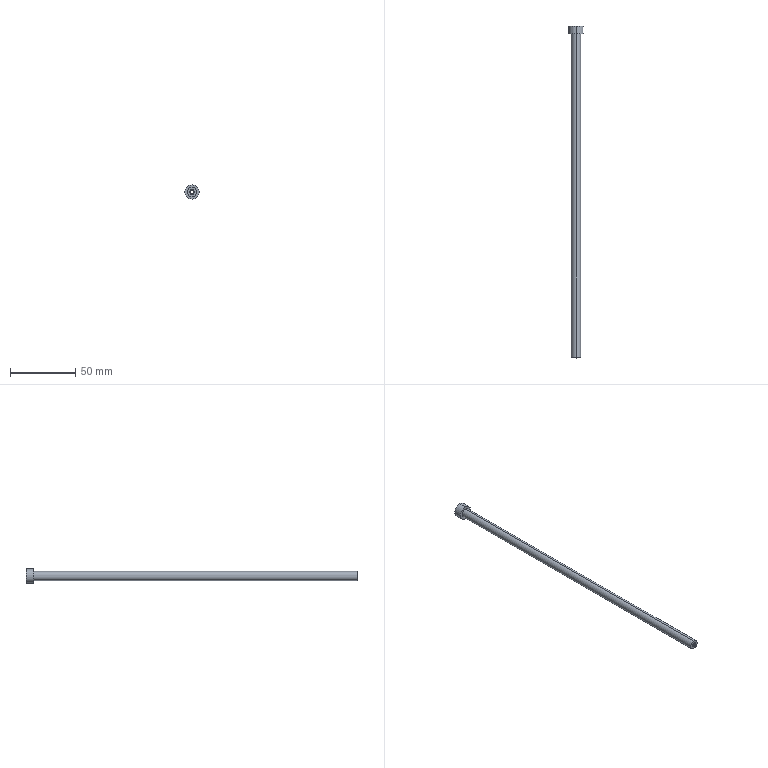Part | STEP file | 1 solid | 13 faces | box 11 x 254.534 x 11 mm | volume 8863 mm3 | cylinder 6 | cone 4 | plane 3 | commonest cylinder face diameters 2.5 x2 7 x2 11 x2
STEP:
#1=CARTESIAN_POINT('',(0.,0.,0.));
#2=DIRECTION('',(0.,0.,1.));
#3=DIRECTION('',(1.,0.,0.));
#4=AXIS2_PLACEMENT_3D('',#1,#2,#3);
#5=CARTESIAN_POINT('',(-16.582,290.5,177.41));
#6=VERTEX_POINT('',#5);
#7=CARTESIAN_POINT('',(-16.582,290.5,188.41));
#8=VERTEX_POINT('',#7);
#9=CARTESIAN_POINT('',(-16.582,290.5,182.91));
#10=DIRECTION('',(0.,-1.,0.));
#11=DIRECTION('',(0.,0.,-1.));
#12=AXIS2_PLACEMENT_3D('',#9,#10,#11);
#13=CIRCLE('',#12,5.5);
#14=CARTESIAN_POINT('',(-16.582,290.5,182.91));
#15=DIRECTION('',(0.,-1.,0.));
#16=DIRECTION('',(0.,0.,-1.));
#17=AXIS2_PLACEMENT_3D('',#14,#15,#16);
#18=CYLINDRICAL_SURFACE('',#17,5.5);
#19=CARTESIAN_POINT('',(0.,0.));
#20=DIRECTION('',(1.,0.));
#21=VECTOR('',#20,1.);
#22=LINE('',#19,#21);
#23=(GEOMETRIC_REPRESENTATION_CONTEXT(2)PARAMETRIC_REPRESENTATION_CONTEXT()REPRESENTATION_CONTEXT('',''));
#24=DEFINITIONAL_REPRESENTATION('',(#22),#23);
#25=PCURVE('',#18,#24);
#26=CARTESIAN_POINT('',(-72.862,290.5,110.196));
#27=DIRECTION('',(0.,-1.,0.));
#28=DIRECTION('',(0.,0.,-1.));
#29=AXIS2_PLACEMENT_3D('',#26,#27,#28);
#30=PLANE('',#29);
#31=CARTESIAN_POINT('',(-72.714,56.28));
#32=DIRECTION('',(1.,0.));
#33=AXIS2_PLACEMENT_2D('',#31,#32);
#34=CIRCLE('',#33,5.5);
#35=(GEOMETRIC_REPRESENTATION_CONTEXT(2)PARAMETRIC_REPRESENTATION_CONTEXT()REPRESENTATION_CONTEXT('',''));
#36=DEFINITIONAL_REPRESENTATION('',(#34),#35);
#37=PCURVE('',#30,#36);
#38=SURFACE_CURVE('',#13,(#25,#37),.PCURVE_S1.);
#39=EDGE_CURVE('',#6,#8,#38,.T.);
#40=ORIENTED_EDGE('',*,*,#39,.T.);
#41=CARTESIAN_POINT('',(-16.582,284.5,188.41));
#42=VERTEX_POINT('',#41);
#43=CARTESIAN_POINT('',(-16.582,290.5,188.41));
#44=DIRECTION('',(0.,-1.,0.));
#45=VECTOR('',#44,1.);
#46=LINE('',#43,#45);
#47=CARTESIAN_POINT('',(3.142,0.));
#48=DIRECTION('',(0.,1.));
#49=VECTOR('',#48,1.);
#50=LINE('',#47,#49);
#51=(GEOMETRIC_REPRESENTATION_CONTEXT(2)PARAMETRIC_REPRESENTATION_CONTEXT()REPRESENTATION_CONTEXT('',''));
#52=DEFINITIONAL_REPRESENTATION('',(#50),#51);
#53=PCURVE('',#18,#52);
#54=CARTESIAN_POINT('',(-16.582,290.5,182.91));
#55=DIRECTION('',(0.,-1.,0.));
#56=DIRECTION('',(0.,0.,-1.));
#57=AXIS2_PLACEMENT_3D('',#54,#55,#56);
#58=CYLINDRICAL_SURFACE('',#57,5.5);
#59=CARTESIAN_POINT('',(3.142,0.));
#60=DIRECTION('',(0.,1.));
#61=VECTOR('',#60,1.);
#62=LINE('',#59,#61);
#63=(GEOMETRIC_REPRESENTATION_CONTEXT(2)PARAMETRIC_REPRESENTATION_CONTEXT()REPRESENTATION_CONTEXT('',''));
#64=DEFINITIONAL_REPRESENTATION('',(#62),#63);
#65=PCURVE('',#58,#64);
#66=SURFACE_CURVE('',#46,(#53,#65),.PCURVE_S1.);
#67=EDGE_CURVE('',#8,#42,#66,.T.);
#68=ORIENTED_EDGE('',*,*,#67,.T.);
#69=CARTESIAN_POINT('',(-16.582,284.5,177.41));
#70=VERTEX_POINT('',#69);
#71=CARTESIAN_POINT('',(-16.582,284.5,182.91));
#72=DIRECTION('',(0.,1.,0.));
#73=DIRECTION('',(0.,0.,1.));
#74=AXIS2_PLACEMENT_3D('',#71,#72,#73);
#75=CIRCLE('',#74,5.5);
#76=CARTESIAN_POINT('',(3.142,6.));
#77=DIRECTION('',(-1.,0.));
#78=VECTOR('',#77,1.);
#79=LINE('',#76,#78);
#80=(GEOMETRIC_REPRESENTATION_CONTEXT(2)PARAMETRIC_REPRESENTATION_CONTEXT()REPRESENTATION_CONTEXT('',''));
#81=DEFINITIONAL_REPRESENTATION('',(#79),#80);
#82=PCURVE('',#18,#81);
#83=CARTESIAN_POINT('',(-16.582,284.5,182.91));
#84=DIRECTION('',(0.,-1.,0.));
#85=DIRECTION('',(0.,0.,-1.));
#86=AXIS2_PLACEMENT_3D('',#83,#84,#85);
#87=PLANE('',#86);
#88=CARTESIAN_POINT('',(-5.5,0.));
#89=CARTESIAN_POINT('',(-5.5,9.526));
#90=CARTESIAN_POINT('',(2.75,4.763));
#91=CARTESIAN_POINT('',(11.,0.));
#92=CARTESIAN_POINT('',(2.75,-4.763));
#93=CARTESIAN_POINT('',(-5.5,-9.526));
#94=CARTESIAN_POINT('',(-5.5,0.));
#95=(BOUNDED_CURVE()B_SPLINE_CURVE(2,(#88,#89,#90,#91,#92,#93,#94),.UNSPECIFIED.,.T.,.F.)B_SPLINE_CURVE_WITH_KNOTS((1,2,2,2,2,1),(-2.094,0.,2.094,4.189,6.283,8.378),.UNSPECIFIED.)CURVE()GEOMETRIC_REPRESENTATION_ITEM()RATIONAL_B_SPLINE_CURVE((1.,0.5,1.,0.5,1.,0.5,1.))REPRESENTATION_ITEM(''));
#96=(GEOMETRIC_REPRESENTATION_CONTEXT(2)PARAMETRIC_REPRESENTATION_CONTEXT()REPRESENTATION_CONTEXT('',''));
#97=DEFINITIONAL_REPRESENTATION('',(#95),#96);
#98=PCURVE('',#87,#97);
#99=SURFACE_CURVE('',#75,(#82,#98),.PCURVE_S1.);
#100=EDGE_CURVE('',#42,#70,#99,.T.);
#101=ORIENTED_EDGE('',*,*,#100,.T.);
#102=CARTESIAN_POINT('',(-16.582,290.5,177.41));
#103=DIRECTION('',(0.,-1.,0.));
#104=VECTOR('',#103,1.);
#105=LINE('',#102,#104);
#106=CARTESIAN_POINT('',(0.,0.));
#107=DIRECTION('',(0.,1.));
#108=VECTOR('',#107,1.);
#109=LINE('',#106,#108);
#110=(GEOMETRIC_REPRESENTATION_CONTEXT(2)PARAMETRIC_REPRESENTATION_CONTEXT()REPRESENTATION_CONTEXT('',''));
#111=DEFINITIONAL_REPRESENTATION('',(#109),#110);
#112=PCURVE('',#18,#111);
#113=CARTESIAN_POINT('',(6.283,0.));
#114=DIRECTION('',(0.,1.));
#115=VECTOR('',#114,1.);
#116=LINE('',#113,#115);
#117=(GEOMETRIC_REPRESENTATION_CONTEXT(2)PARAMETRIC_REPRESENTATION_CONTEXT()REPRESENTATION_CONTEXT('',''));
#118=DEFINITIONAL_REPRESENTATION('',(#116),#117);
#119=PCURVE('',#58,#118);
#120=SURFACE_CURVE('',#105,(#112,#119),.PCURVE_S1.);
#121=EDGE_CURVE('',#6,#70,#120,.T.);
#122=ORIENTED_EDGE('',*,*,#121,.F.);
#123=EDGE_LOOP('',(#40,#68,#101,#122));
#124=FACE_BOUND('',#123,.T.);
#125=ADVANCED_FACE('',(#124),#18,.T.);
#126=CARTESIAN_POINT('',(-16.582,35.966,184.16));
#127=VERTEX_POINT('',#126);
#128=CARTESIAN_POINT('',(-16.582,290.5,184.16));
#129=VERTEX_POINT('',#128);
#130=CARTESIAN_POINT('',(-16.582,27.637,184.16));
#131=DIRECTION('',(0.,1.,0.));
#132=VECTOR('',#131,1.);
#133=LINE('',#130,#132);
#134=CARTESIAN_POINT('',(-16.582,27.637,182.91));
#135=DIRECTION('',(0.,1.,0.));
#136=DIRECTION('',(0.,0.,1.));
#137=AXIS2_PLACEMENT_3D('',#134,#135,#136);
#138=CYLINDRICAL_SURFACE('',#137,1.25);
#139=CARTESIAN_POINT('',(6.283,0.));
#140=DIRECTION('',(0.,1.));
#141=VECTOR('',#140,1.);
#142=LINE('',#139,#141);
#143=(GEOMETRIC_REPRESENTATION_CONTEXT(2)PARAMETRIC_REPRESENTATION_CONTEXT()REPRESENTATION_CONTEXT('',''));
#144=DEFINITIONAL_REPRESENTATION('',(#142),#143);
#145=PCURVE('',#138,#144);
#146=CARTESIAN_POINT('',(-16.582,27.637,182.91));
#147=DIRECTION('',(0.,1.,0.));
#148=DIRECTION('',(0.,0.,1.));
#149=AXIS2_PLACEMENT_3D('',#146,#147,#148);
#150=CYLINDRICAL_SURFACE('',#149,1.25);
#151=CARTESIAN_POINT('',(0.,0.));
#152=DIRECTION('',(0.,1.));
#153=VECTOR('',#152,1.);
#154=LINE('',#151,#153);
#155=(GEOMETRIC_REPRESENTATION_CONTEXT(2)PARAMETRIC_REPRESENTATION_CONTEXT()REPRESENTATION_CONTEXT('',''));
#156=DEFINITIONAL_REPRESENTATION('',(#154),#155);
#157=PCURVE('',#150,#156);
#158=SURFACE_CURVE('',#133,(#145,#157),.PCURVE_S1.);
#159=EDGE_CURVE('',#127,#129,#158,.T.);
#160=ORIENTED_EDGE('',*,*,#159,.T.);
#161=CARTESIAN_POINT('',(-16.582,290.5,181.66));
#162=VERTEX_POINT('',#161);
#163=CARTESIAN_POINT('',(-16.582,290.5,182.91));
#164=DIRECTION('',(0.,-1.,0.));
#165=DIRECTION('',(0.,0.,-1.));
#166=AXIS2_PLACEMENT_3D('',#163,#164,#165);
#167=CIRCLE('',#166,1.25);
#168=CARTESIAN_POINT('',(9.425,262.863));
#169=DIRECTION('',(-1.,0.));
#170=VECTOR('',#169,1.);
#171=LINE('',#168,#170);
#172=(GEOMETRIC_REPRESENTATION_CONTEXT(2)PARAMETRIC_REPRESENTATION_CONTEXT()REPRESENTATION_CONTEXT('',''));
#173=DEFINITIONAL_REPRESENTATION('',(#171),#172);
#174=PCURVE('',#138,#173);
#175=CARTESIAN_POINT('',(-72.714,56.28));
#176=DIRECTION('',(1.,0.));
#177=AXIS2_PLACEMENT_2D('',#175,#176);
#178=CIRCLE('',#177,1.25);
#179=(GEOMETRIC_REPRESENTATION_CONTEXT(2)PARAMETRIC_REPRESENTATION_CONTEXT()REPRESENTATION_CONTEXT('',''));
#180=DEFINITIONAL_REPRESENTATION('',(#178),#179);
#181=PCURVE('',#30,#180);
#182=SURFACE_CURVE('',#167,(#174,#181),.PCURVE_S1.);
#183=EDGE_CURVE('',#129,#162,#182,.T.);
#184=ORIENTED_EDGE('',*,*,#183,.T.);
#185=CARTESIAN_POINT('',(-16.582,35.966,181.66));
#186=VERTEX_POINT('',#185);
#187=CARTESIAN_POINT('',(-16.582,27.637,181.66));
#188=DIRECTION('',(0.,1.,0.));
#189=VECTOR('',#188,1.);
#190=LINE('',#187,#189);
#191=CARTESIAN_POINT('',(3.142,0.));
#192=DIRECTION('',(0.,1.));
#193=VECTOR('',#192,1.);
#194=LINE('',#191,#193);
#195=(GEOMETRIC_REPRESENTATION_CONTEXT(2)PARAMETRIC_REPRESENTATION_CONTEXT()REPRESENTATION_CONTEXT('',''));
#196=DEFINITIONAL_REPRESENTATION('',(#194),#195);
#197=PCURVE('',#138,#196);
#198=CARTESIAN_POINT('',(3.142,0.));
#199=DIRECTION('',(0.,1.));
#200=VECTOR('',#199,1.);
#201=LINE('',#198,#200);
#202=(GEOMETRIC_REPRESENTATION_CONTEXT(2)PARAMETRIC_REPRESENTATION_CONTEXT()REPRESENTATION_CONTEXT('',''));
#203=DEFINITIONAL_REPRESENTATION('',(#201),#202);
#204=PCURVE('',#150,#203);
#205=SURFACE_CURVE('',#190,(#197,#204),.PCURVE_S1.);
#206=EDGE_CURVE('',#186,#162,#205,.T.);
#207=ORIENTED_EDGE('',*,*,#206,.F.);
#208=CARTESIAN_POINT('',(-16.582,35.966,182.91));
#209=DIRECTION('',(0.,1.,0.));
#210=DIRECTION('',(0.,0.,1.));
#211=AXIS2_PLACEMENT_3D('',#208,#209,#210);
#212=CIRCLE('',#211,1.25);
#213=CARTESIAN_POINT('',(0.,8.329));
#214=DIRECTION('',(1.,0.));
#215=VECTOR('',#214,1.);
#216=LINE('',#213,#215);
#217=(GEOMETRIC_REPRESENTATION_CONTEXT(2)PARAMETRIC_REPRESENTATION_CONTEXT()REPRESENTATION_CONTEXT('',''));
#218=DEFINITIONAL_REPRESENTATION('',(#216),#217);
#219=PCURVE('',#138,#218);
#220=CARTESIAN_POINT('',(-16.582,36.682,182.91));
#221=DIRECTION('',(0.,1.,0.));
#222=DIRECTION('',(0.,0.,1.));
#223=AXIS2_PLACEMENT_3D('',#220,#221,#222);
#224=CONICAL_SURFACE('',#223,1.256,0.008727);
#225=CARTESIAN_POINT('',(0.,-0.7162));
#226=DIRECTION('',(1.,0.));
#227=VECTOR('',#226,1.);
#228=LINE('',#225,#227);
#229=(GEOMETRIC_REPRESENTATION_CONTEXT(2)PARAMETRIC_REPRESENTATION_CONTEXT()REPRESENTATION_CONTEXT('',''));
#230=DEFINITIONAL_REPRESENTATION('',(#228),#229);
#231=PCURVE('',#224,#230);
#232=SURFACE_CURVE('',#212,(#219,#231),.PCURVE_S1.);
#233=EDGE_CURVE('',#186,#127,#232,.T.);
#234=ORIENTED_EDGE('',*,*,#233,.T.);
#235=EDGE_LOOP('',(#160,#184,#207,#234));
#236=FACE_BOUND('',#235,.F.);
#237=ADVANCED_FACE('',(#236),#138,.F.);
#238=CARTESIAN_POINT('',(-16.582,36.682,179.41));
#239=VERTEX_POINT('',#238);
#240=CARTESIAN_POINT('',(-16.582,36.682,186.41));
#241=VERTEX_POINT('',#240);
#242=CARTESIAN_POINT('',(-16.582,36.682,182.91));
#243=DIRECTION('',(0.,-1.,0.));
#244=DIRECTION('',(0.,0.,1.));
#245=AXIS2_PLACEMENT_3D('',#242,#243,#244);
#246=CIRCLE('',#245,3.5);
#247=CARTESIAN_POINT('',(-16.582,27.637,182.91));
#248=DIRECTION('',(0.,1.,0.));
#249=DIRECTION('',(0.,0.,1.));
#250=AXIS2_PLACEMENT_3D('',#247,#248,#249);
#251=CYLINDRICAL_SURFACE('',#250,3.5);
#252=CARTESIAN_POINT('',(6.283,9.045));
#253=DIRECTION('',(-1.,0.));
#254=VECTOR('',#253,1.);
#255=LINE('',#252,#254);
#256=(GEOMETRIC_REPRESENTATION_CONTEXT(2)PARAMETRIC_REPRESENTATION_CONTEXT()REPRESENTATION_CONTEXT('',''));
#257=DEFINITIONAL_REPRESENTATION('',(#255),#256);
#258=PCURVE('',#251,#257);
#259=CARTESIAN_POINT('',(-16.582,36.682,182.91));
#260=DIRECTION('',(0.,1.,0.));
#261=DIRECTION('',(0.,0.,1.));
#262=AXIS2_PLACEMENT_3D('',#259,#260,#261);
#263=PLANE('',#262);
#264=CARTESIAN_POINT('',(3.5,0.));
#265=CARTESIAN_POINT('',(3.5,-6.062));
#266=CARTESIAN_POINT('',(-1.75,-3.031));
#267=CARTESIAN_POINT('',(-7.,0.));
#268=CARTESIAN_POINT('',(-1.75,3.031));
#269=CARTESIAN_POINT('',(3.5,6.062));
#270=CARTESIAN_POINT('',(3.5,0.));
#271=(BOUNDED_CURVE()B_SPLINE_CURVE(2,(#264,#265,#266,#267,#268,#269,#270),.UNSPECIFIED.,.T.,.F.)B_SPLINE_CURVE_WITH_KNOTS((1,2,2,2,2,1),(-2.094,0.,2.094,4.189,6.283,8.378),.UNSPECIFIED.)CURVE()GEOMETRIC_REPRESENTATION_ITEM()RATIONAL_B_SPLINE_CURVE((1.,0.5,1.,0.5,1.,0.5,1.))REPRESENTATION_ITEM(''));
#272=(GEOMETRIC_REPRESENTATION_CONTEXT(2)PARAMETRIC_REPRESENTATION_CONTEXT()REPRESENTATION_CONTEXT('',''));
#273=DEFINITIONAL_REPRESENTATION('',(#271),#272);
#274=PCURVE('',#263,#273);
#275=SURFACE_CURVE('',#246,(#258,#274),.PCURVE_S1.);
#276=EDGE_CURVE('',#239,#241,#275,.T.);
#277=ORIENTED_EDGE('',*,*,#276,.F.);
#278=CARTESIAN_POINT('',(-16.582,284.5,179.41));
#279=VERTEX_POINT('',#278);
#280=CARTESIAN_POINT('',(-16.582,27.637,179.41));
#281=DIRECTION('',(0.,1.,0.));
#282=VECTOR('',#281,1.);
#283=LINE('',#280,#282);
#284=CARTESIAN_POINT('',(3.142,0.));
#285=DIRECTION('',(0.,1.));
#286=VECTOR('',#285,1.);
#287=LINE('',#284,#286);
#288=(GEOMETRIC_REPRESENTATION_CONTEXT(2)PARAMETRIC_REPRESENTATION_CONTEXT()REPRESENTATION_CONTEXT('',''));
#289=DEFINITIONAL_REPRESENTATION('',(#287),#288);
#290=PCURVE('',#251,#289);
#291=CARTESIAN_POINT('',(-16.582,27.637,182.91));
#292=DIRECTION('',(0.,1.,0.));
#293=DIRECTION('',(0.,0.,1.));
#294=AXIS2_PLACEMENT_3D('',#291,#292,#293);
#295=CYLINDRICAL_SURFACE('',#294,3.5);
#296=CARTESIAN_POINT('',(3.142,0.));
#297=DIRECTION('',(0.,1.));
#298=VECTOR('',#297,1.);
#299=LINE('',#296,#298);
#300=(GEOMETRIC_REPRESENTATION_CONTEXT(2)PARAMETRIC_REPRESENTATION_CONTEXT()REPRESENTATION_CONTEXT('',''));
#301=DEFINITIONAL_REPRESENTATION('',(#299),#300);
#302=PCURVE('',#295,#301);
#303=SURFACE_CURVE('',#283,(#290,#302),.PCURVE_S1.);
#304=EDGE_CURVE('',#239,#279,#303,.T.);
#305=ORIENTED_EDGE('',*,*,#304,.T.);
#306=CARTESIAN_POINT('',(-16.582,284.5,186.41));
#307=VERTEX_POINT('',#306);
#308=CARTESIAN_POINT('',(-16.582,284.5,182.91));
#309=DIRECTION('',(0.,1.,0.));
#310=DIRECTION('',(0.,0.,-1.));
#311=AXIS2_PLACEMENT_3D('',#308,#309,#310);
#312=CIRCLE('',#311,3.5);
#313=CARTESIAN_POINT('',(-3.142,256.863));
#314=DIRECTION('',(1.,0.));
#315=VECTOR('',#314,1.);
#316=LINE('',#313,#315);
#317=(GEOMETRIC_REPRESENTATION_CONTEXT(2)PARAMETRIC_REPRESENTATION_CONTEXT()REPRESENTATION_CONTEXT('',''));
#318=DEFINITIONAL_REPRESENTATION('',(#316),#317);
#319=PCURVE('',#251,#318);
#320=CARTESIAN_POINT('',(3.5,0.));
#321=CARTESIAN_POINT('',(3.5,-6.062));
#322=CARTESIAN_POINT('',(-1.75,-3.031));
#323=CARTESIAN_POINT('',(-7.,0.));
#324=CARTESIAN_POINT('',(-1.75,3.031));
#325=CARTESIAN_POINT('',(3.5,6.062));
#326=CARTESIAN_POINT('',(3.5,0.));
#327=(BOUNDED_CURVE()B_SPLINE_CURVE(2,(#320,#321,#322,#323,#324,#325,#326),.UNSPECIFIED.,.T.,.F.)B_SPLINE_CURVE_WITH_KNOTS((1,2,2,2,2,1),(-2.094,0.,2.094,4.189,6.283,8.378),.UNSPECIFIED.)CURVE()GEOMETRIC_REPRESENTATION_ITEM()RATIONAL_B_SPLINE_CURVE((1.,0.5,1.,0.5,1.,0.5,1.))REPRESENTATION_ITEM(''));
#328=(GEOMETRIC_REPRESENTATION_CONTEXT(2)PARAMETRIC_REPRESENTATION_CONTEXT()REPRESENTATION_CONTEXT('',''));
#329=DEFINITIONAL_REPRESENTATION('',(#327),#328);
#330=PCURVE('',#87,#329);
#331=SURFACE_CURVE('',#312,(#319,#330),.PCURVE_S1.);
#332=EDGE_CURVE('',#307,#279,#331,.T.);
#333=ORIENTED_EDGE('',*,*,#332,.F.);
#334=CARTESIAN_POINT('',(-16.582,27.637,186.41));
#335=DIRECTION('',(0.,1.,0.));
#336=VECTOR('',#335,1.);
#337=LINE('',#334,#336);
#338=CARTESIAN_POINT('',(0.,0.));
#339=DIRECTION('',(0.,1.));
#340=VECTOR('',#339,1.);
#341=LINE('',#338,#340);
#342=(GEOMETRIC_REPRESENTATION_CONTEXT(2)PARAMETRIC_REPRESENTATION_CONTEXT()REPRESENTATION_CONTEXT('',''));
#343=DEFINITIONAL_REPRESENTATION('',(#341),#342);
#344=PCURVE('',#251,#343);
#345=CARTESIAN_POINT('',(6.283,0.));
#346=DIRECTION('',(0.,1.));
#347=VECTOR('',#346,1.);
#348=LINE('',#345,#347);
#349=(GEOMETRIC_REPRESENTATION_CONTEXT(2)PARAMETRIC_REPRESENTATION_CONTEXT()REPRESENTATION_CONTEXT('',''));
#350=DEFINITIONAL_REPRESENTATION('',(#348),#349);
#351=PCURVE('',#295,#350);
#352=SURFACE_CURVE('',#337,(#344,#351),.PCURVE_S1.);
#353=EDGE_CURVE('',#241,#307,#352,.T.);
#354=ORIENTED_EDGE('',*,*,#353,.F.);
#355=EDGE_LOOP('',(#277,#305,#333,#354));
#356=FACE_BOUND('',#355,.T.);
#357=ADVANCED_FACE('',(#356),#251,.T.);
#358=CARTESIAN_POINT('',(-16.582,36.176,184.162));
#359=VERTEX_POINT('',#358);
#360=CARTESIAN_POINT('',(-16.582,36.176,181.658));
#361=VERTEX_POINT('',#360);
#362=CARTESIAN_POINT('',(-16.582,36.176,182.91));
#363=DIRECTION('',(0.,1.,0.));
#364=DIRECTION('',(0.,0.,1.));
#365=AXIS2_PLACEMENT_3D('',#362,#363,#364);
#366=CIRCLE('',#365,1.252);
#367=CARTESIAN_POINT('',(-16.582,36.176,182.91));
#368=DIRECTION('',(0.,1.,0.));
#369=DIRECTION('',(0.,0.,1.));
#370=AXIS2_PLACEMENT_3D('',#367,#368,#369);
#371=CONICAL_SURFACE('',#370,1.252,0.7854);
#372=CARTESIAN_POINT('',(0.,0.));
#373=DIRECTION('',(1.,0.));
#374=VECTOR('',#373,1.);
#375=LINE('',#372,#374);
#376=(GEOMETRIC_REPRESENTATION_CONTEXT(2)PARAMETRIC_REPRESENTATION_CONTEXT()REPRESENTATION_CONTEXT('',''));
#377=DEFINITIONAL_REPRESENTATION('',(#375),#376);
#378=PCURVE('',#371,#377);
#379=CARTESIAN_POINT('',(-16.582,36.682,182.91));
#380=DIRECTION('',(0.,1.,0.));
#381=DIRECTION('',(0.,0.,1.));
#382=AXIS2_PLACEMENT_3D('',#379,#380,#381);
#383=CONICAL_SURFACE('',#382,1.256,0.008727);
#384=CARTESIAN_POINT('',(0.,-0.5069));
#385=DIRECTION('',(1.,0.));
#386=VECTOR('',#385,1.);
#387=LINE('',#384,#386);
#388=(GEOMETRIC_REPRESENTATION_CONTEXT(2)PARAMETRIC_REPRESENTATION_CONTEXT()REPRESENTATION_CONTEXT('',''));
#389=DEFINITIONAL_REPRESENTATION('',(#387),#388);
#390=PCURVE('',#383,#389);
#391=SURFACE_CURVE('',#366,(#378,#390),.PCURVE_S1.);
#392=EDGE_CURVE('',#359,#361,#391,.T.);
#393=ORIENTED_EDGE('',*,*,#392,.T.);
#394=CARTESIAN_POINT('',(-16.582,36.682,181.151));
#395=VERTEX_POINT('',#394);
#396=CARTESIAN_POINT('',(-16.582,36.176,181.658));
#397=DIRECTION('',(0.,0.7071,-0.7071));
#398=VECTOR('',#397,1.);
#399=LINE('',#396,#398);
#400=CARTESIAN_POINT('',(3.142,0.));
#401=DIRECTION('',(0.,1.));
#402=VECTOR('',#401,1.);
#403=LINE('',#400,#402);
#404=(GEOMETRIC_REPRESENTATION_CONTEXT(2)PARAMETRIC_REPRESENTATION_CONTEXT()REPRESENTATION_CONTEXT('',''));
#405=DEFINITIONAL_REPRESENTATION('',(#403),#404);
#406=PCURVE('',#371,#405);
#407=CARTESIAN_POINT('',(-16.582,36.176,182.91));
#408=DIRECTION('',(0.,1.,0.));
#409=DIRECTION('',(0.,0.,1.));
#410=AXIS2_PLACEMENT_3D('',#407,#408,#409);
#411=CONICAL_SURFACE('',#410,1.252,0.7854);
#412=CARTESIAN_POINT('',(3.142,0.));
#413=DIRECTION('',(0.,1.));
#414=VECTOR('',#413,1.);
#415=LINE('',#412,#414);
#416=(GEOMETRIC_REPRESENTATION_CONTEXT(2)PARAMETRIC_REPRESENTATION_CONTEXT()REPRESENTATION_CONTEXT('',''));
#417=DEFINITIONAL_REPRESENTATION('',(#415),#416);
#418=PCURVE('',#411,#417);
#419=SURFACE_CURVE('',#399,(#406,#418),.PCURVE_S1.);
#420=EDGE_CURVE('',#361,#395,#419,.T.);
#421=ORIENTED_EDGE('',*,*,#420,.T.);
#422=CARTESIAN_POINT('',(-16.582,36.682,184.669));
#423=VERTEX_POINT('',#422);
#424=CARTESIAN_POINT('',(-16.582,36.682,182.91));
#425=DIRECTION('',(0.,-1.,0.));
#426=DIRECTION('',(0.,0.,1.));
#427=AXIS2_PLACEMENT_3D('',#424,#425,#426);
#428=CIRCLE('',#427,1.759);
#429=CARTESIAN_POINT('',(6.283,0.5069));
#430=DIRECTION('',(-1.,0.));
#431=VECTOR('',#430,1.);
#432=LINE('',#429,#431);
#433=(GEOMETRIC_REPRESENTATION_CONTEXT(2)PARAMETRIC_REPRESENTATION_CONTEXT()REPRESENTATION_CONTEXT('',''));
#434=DEFINITIONAL_REPRESENTATION('',(#432),#433);
#435=PCURVE('',#371,#434);
#436=CARTESIAN_POINT('',(1.759,0.));
#437=CARTESIAN_POINT('',(1.759,-3.046));
#438=CARTESIAN_POINT('',(-0.8794,-1.523));
#439=CARTESIAN_POINT('',(-3.518,0.));
#440=CARTESIAN_POINT('',(-0.8794,1.523));
#441=CARTESIAN_POINT('',(1.759,3.046));
#442=CARTESIAN_POINT('',(1.759,0.));
#443=(BOUNDED_CURVE()B_SPLINE_CURVE(2,(#436,#437,#438,#439,#440,#441,#442),.UNSPECIFIED.,.T.,.F.)B_SPLINE_CURVE_WITH_KNOTS((1,2,2,2,2,1),(-2.094,0.,2.094,4.189,6.283,8.378),.UNSPECIFIED.)CURVE()GEOMETRIC_REPRESENTATION_ITEM()RATIONAL_B_SPLINE_CURVE((1.,0.5,1.,0.5,1.,0.5,1.))REPRESENTATION_ITEM(''));
#444=(GEOMETRIC_REPRESENTATION_CONTEXT(2)PARAMETRIC_REPRESENTATION_CONTEXT()REPRESENTATION_CONTEXT('',''));
#445=DEFINITIONAL_REPRESENTATION('',(#443),#444);
#446=PCURVE('',#263,#445);
#447=SURFACE_CURVE('',#428,(#435,#446),.PCURVE_S1.);
#448=EDGE_CURVE('',#395,#423,#447,.T.);
#449=ORIENTED_EDGE('',*,*,#448,.T.);
#450=CARTESIAN_POINT('',(-16.582,36.176,184.162));
#451=DIRECTION('',(0.,0.7071,0.7071));
#452=VECTOR('',#451,1.);
#453=LINE('',#450,#452);
#454=CARTESIAN_POINT('',(0.,0.));
#455=DIRECTION('',(0.,1.));
#456=VECTOR('',#455,1.);
#457=LINE('',#454,#456);
#458=(GEOMETRIC_REPRESENTATION_CONTEXT(2)PARAMETRIC_REPRESENTATION_CONTEXT()REPRESENTATION_CONTEXT('',''));
#459=DEFINITIONAL_REPRESENTATION('',(#457),#458);
#460=PCURVE('',#371,#459);
#461=CARTESIAN_POINT('',(6.283,0.));
#462=DIRECTION('',(0.,1.));
#463=VECTOR('',#462,1.);
#464=LINE('',#461,#463);
#465=(GEOMETRIC_REPRESENTATION_CONTEXT(2)PARAMETRIC_REPRESENTATION_CONTEXT()REPRESENTATION_CONTEXT('',''));
#466=DEFINITIONAL_REPRESENTATION('',(#464),#465);
#467=PCURVE('',#411,#466);
#468=SURFACE_CURVE('',#453,(#460,#467),.PCURVE_S1.);
#469=EDGE_CURVE('',#359,#423,#468,.T.);
#470=ORIENTED_EDGE('',*,*,#469,.F.);
#471=EDGE_LOOP('',(#393,#421,#449,#470));
#472=FACE_BOUND('',#471,.T.);
#473=ADVANCED_FACE('',(#472),#371,.T.);
#474=CARTESIAN_POINT('',(-16.582,35.966,182.91));
#475=DIRECTION('',(0.,1.,0.));
#476=DIRECTION('',(0.,0.,1.));
#477=AXIS2_PLACEMENT_3D('',#474,#475,#476);
#478=CIRCLE('',#477,1.25);
#479=CARTESIAN_POINT('',(0.,-0.7162));
#480=DIRECTION('',(1.,0.));
#481=VECTOR('',#480,1.);
#482=LINE('',#479,#481);
#483=(GEOMETRIC_REPRESENTATION_CONTEXT(2)PARAMETRIC_REPRESENTATION_CONTEXT()REPRESENTATION_CONTEXT('',''));
#484=DEFINITIONAL_REPRESENTATION('',(#482),#483);
#485=PCURVE('',#383,#484);
#486=CARTESIAN_POINT('',(0.,8.329));
#487=DIRECTION('',(1.,0.));
#488=VECTOR('',#487,1.);
#489=LINE('',#486,#488);
#490=(GEOMETRIC_REPRESENTATION_CONTEXT(2)PARAMETRIC_REPRESENTATION_CONTEXT()REPRESENTATION_CONTEXT('',''));
#491=DEFINITIONAL_REPRESENTATION('',(#489),#490);
#492=PCURVE('',#150,#491);
#493=SURFACE_CURVE('',#478,(#485,#492),.PCURVE_S1.);
#494=EDGE_CURVE('',#127,#186,#493,.T.);
#495=ORIENTED_EDGE('',*,*,#494,.T.);
#496=CARTESIAN_POINT('',(-16.582,36.682,181.654));
#497=DIRECTION('',(0.,1.,-0.008727));
#498=VECTOR('',#497,1.);
#499=LINE('',#496,#498);
#500=CARTESIAN_POINT('',(3.142,0.));
#501=DIRECTION('',(0.,1.));
#502=VECTOR('',#501,1.);
#503=LINE('',#500,#502);
#504=(GEOMETRIC_REPRESENTATION_CONTEXT(2)PARAMETRIC_REPRESENTATION_CONTEXT()REPRESENTATION_CONTEXT('',''));
#505=DEFINITIONAL_REPRESENTATION('',(#503),#504);
#506=PCURVE('',#383,#505);
#507=CARTESIAN_POINT('',(3.142,0.));
#508=DIRECTION('',(0.,1.));
#509=VECTOR('',#508,1.);
#510=LINE('',#507,#509);
#511=(GEOMETRIC_REPRESENTATION_CONTEXT(2)PARAMETRIC_REPRESENTATION_CONTEXT()REPRESENTATION_CONTEXT('',''));
#512=DEFINITIONAL_REPRESENTATION('',(#510),#511);
#513=PCURVE('',#224,#512);
#514=SURFACE_CURVE('',#499,(#506,#513),.PCURVE_S1.);
#515=EDGE_CURVE('',#186,#361,#514,.T.);
#516=ORIENTED_EDGE('',*,*,#515,.T.);
#517=ORIENTED_EDGE('',*,*,#392,.F.);
#518=CARTESIAN_POINT('',(-16.582,36.682,184.166));
#519=DIRECTION('',(0.,1.,0.008727));
#520=VECTOR('',#519,1.);
#521=LINE('',#518,#520);
#522=CARTESIAN_POINT('',(0.,0.));
#523=DIRECTION('',(0.,1.));
#524=VECTOR('',#523,1.);
#525=LINE('',#522,#524);
#526=(GEOMETRIC_REPRESENTATION_CONTEXT(2)PARAMETRIC_REPRESENTATION_CONTEXT()REPRESENTATION_CONTEXT('',''));
#527=DEFINITIONAL_REPRESENTATION('',(#525),#526);
#528=PCURVE('',#383,#527);
#529=CARTESIAN_POINT('',(6.283,0.));
#530=DIRECTION('',(0.,1.));
#531=VECTOR('',#530,1.);
#532=LINE('',#529,#531);
#533=(GEOMETRIC_REPRESENTATION_CONTEXT(2)PARAMETRIC_REPRESENTATION_CONTEXT()REPRESENTATION_CONTEXT('',''));
#534=DEFINITIONAL_REPRESENTATION('',(#532),#533);
#535=PCURVE('',#224,#534);
#536=SURFACE_CURVE('',#521,(#528,#535),.PCURVE_S1.);
#537=EDGE_CURVE('',#127,#359,#536,.T.);
#538=ORIENTED_EDGE('',*,*,#537,.F.);
#539=EDGE_LOOP('',(#495,#516,#517,#538));
#540=FACE_BOUND('',#539,.T.);
#541=ADVANCED_FACE('',(#540),#383,.T.);
#542=ORIENTED_EDGE('',*,*,#515,.F.);
#543=ORIENTED_EDGE('',*,*,#233,.T.);
#544=ORIENTED_EDGE('',*,*,#537,.T.);
#545=CARTESIAN_POINT('',(-16.582,36.176,182.91));
#546=DIRECTION('',(0.,1.,0.));
#547=DIRECTION('',(0.,0.,1.));
#548=AXIS2_PLACEMENT_3D('',#545,#546,#547);
#549=CIRCLE('',#548,1.252);
#550=CARTESIAN_POINT('',(0.,-0.5069));
#551=DIRECTION('',(1.,0.));
#552=VECTOR('',#551,1.);
#553=LINE('',#550,#552);
#554=(GEOMETRIC_REPRESENTATION_CONTEXT(2)PARAMETRIC_REPRESENTATION_CONTEXT()REPRESENTATION_CONTEXT('',''));
#555=DEFINITIONAL_REPRESENTATION('',(#553),#554);
#556=PCURVE('',#224,#555);
#557=CARTESIAN_POINT('',(0.,0.));
#558=DIRECTION('',(1.,0.));
#559=VECTOR('',#558,1.);
#560=LINE('',#557,#559);
#561=(GEOMETRIC_REPRESENTATION_CONTEXT(2)PARAMETRIC_REPRESENTATION_CONTEXT()REPRESENTATION_CONTEXT('',''));
#562=DEFINITIONAL_REPRESENTATION('',(#560),#561);
#563=PCURVE('',#411,#562);
#564=SURFACE_CURVE('',#549,(#556,#563),.PCURVE_S1.);
#565=EDGE_CURVE('',#361,#359,#564,.T.);
#566=ORIENTED_EDGE('',*,*,#565,.F.);
#567=EDGE_LOOP('',(#542,#543,#544,#566));
#568=FACE_BOUND('',#567,.T.);
#569=ADVANCED_FACE('',(#568),#224,.T.);
#570=ORIENTED_EDGE('',*,*,#420,.F.);
#571=ORIENTED_EDGE('',*,*,#565,.T.);
#572=ORIENTED_EDGE('',*,*,#469,.T.);
#573=CARTESIAN_POINT('',(-16.582,36.682,182.91));
#574=DIRECTION('',(0.,-1.,0.));
#575=DIRECTION('',(0.,0.,1.));
#576=AXIS2_PLACEMENT_3D('',#573,#574,#575);
#577=CIRCLE('',#576,1.759);
#578=CARTESIAN_POINT('',(6.283,0.5069));
#579=DIRECTION('',(-1.,0.));
#580=VECTOR('',#579,1.);
#581=LINE('',#578,#580);
#582=(GEOMETRIC_REPRESENTATION_CONTEXT(2)PARAMETRIC_REPRESENTATION_CONTEXT()REPRESENTATION_CONTEXT('',''));
#583=DEFINITIONAL_REPRESENTATION('',(#581),#582);
#584=PCURVE('',#411,#583);
#585=CARTESIAN_POINT('',(1.759,0.));
#586=CARTESIAN_POINT('',(1.759,-3.046));
#587=CARTESIAN_POINT('',(-0.8794,-1.523));
#588=CARTESIAN_POINT('',(-3.518,0.));
#589=CARTESIAN_POINT('',(-0.8794,1.523));
#590=CARTESIAN_POINT('',(1.759,3.046));
#591=CARTESIAN_POINT('',(1.759,0.));
#592=(BOUNDED_CURVE()B_SPLINE_CURVE(2,(#585,#586,#587,#588,#589,#590,#591),.UNSPECIFIED.,.T.,.F.)B_SPLINE_CURVE_WITH_KNOTS((1,2,2,2,2,1),(-2.094,0.,2.094,4.189,6.283,8.378),.UNSPECIFIED.)CURVE()GEOMETRIC_REPRESENTATION_ITEM()RATIONAL_B_SPLINE_CURVE((1.,0.5,1.,0.5,1.,0.5,1.))REPRESENTATION_ITEM(''));
#593=(GEOMETRIC_REPRESENTATION_CONTEXT(2)PARAMETRIC_REPRESENTATION_CONTEXT()REPRESENTATION_CONTEXT('',''));
#594=DEFINITIONAL_REPRESENTATION('',(#592),#593);
#595=PCURVE('',#263,#594);
#596=SURFACE_CURVE('',#577,(#584,#595),.PCURVE_S1.);
#597=EDGE_CURVE('',#423,#395,#596,.T.);
#598=ORIENTED_EDGE('',*,*,#597,.T.);
#599=EDGE_LOOP('',(#570,#571,#572,#598));
#600=FACE_BOUND('',#599,.T.);
#601=ADVANCED_FACE('',(#600),#411,.T.);
#602=CARTESIAN_POINT('',(-16.582,36.682,182.91));
#603=DIRECTION('',(0.,-1.,0.));
#604=DIRECTION('',(0.,0.,1.));
#605=AXIS2_PLACEMENT_3D('',#602,#603,#604);
#606=CIRCLE('',#605,3.5);
#607=CARTESIAN_POINT('',(3.5,0.));
#608=CARTESIAN_POINT('',(3.5,-6.062));
#609=CARTESIAN_POINT('',(-1.75,-3.031));
#610=CARTESIAN_POINT('',(-7.,0.));
#611=CARTESIAN_POINT('',(-1.75,3.031));
#612=CARTESIAN_POINT('',(3.5,6.062));
#613=CARTESIAN_POINT('',(3.5,0.));
#614=(BOUNDED_CURVE()B_SPLINE_CURVE(2,(#607,#608,#609,#610,#611,#612,#613),.UNSPECIFIED.,.T.,.F.)B_SPLINE_CURVE_WITH_KNOTS((1,2,2,2,2,1),(-2.094,0.,2.094,4.189,6.283,8.378),.UNSPECIFIED.)CURVE()GEOMETRIC_REPRESENTATION_ITEM()RATIONAL_B_SPLINE_CURVE((1.,0.5,1.,0.5,1.,0.5,1.))REPRESENTATION_ITEM(''));
#615=(GEOMETRIC_REPRESENTATION_CONTEXT(2)PARAMETRIC_REPRESENTATION_CONTEXT()REPRESENTATION_CONTEXT('',''));
#616=DEFINITIONAL_REPRESENTATION('',(#614),#615);
#617=PCURVE('',#263,#616);
#618=CARTESIAN_POINT('',(6.283,9.045));
#619=DIRECTION('',(-1.,0.));
#620=VECTOR('',#619,1.);
#621=LINE('',#618,#620);
#622=(GEOMETRIC_REPRESENTATION_CONTEXT(2)PARAMETRIC_REPRESENTATION_CONTEXT()REPRESENTATION_CONTEXT('',''));
#623=DEFINITIONAL_REPRESENTATION('',(#621),#622);
#624=PCURVE('',#295,#623);
#625=SURFACE_CURVE('',#606,(#617,#624),.PCURVE_S1.);
#626=EDGE_CURVE('',#241,#239,#625,.T.);
#627=ORIENTED_EDGE('',*,*,#626,.T.);
#628=ORIENTED_EDGE('',*,*,#276,.T.);
#629=EDGE_LOOP('',(#627,#628));
#630=FACE_BOUND('',#629,.T.);
#631=ORIENTED_EDGE('',*,*,#597,.F.);
#632=ORIENTED_EDGE('',*,*,#448,.F.);
#633=EDGE_LOOP('',(#631,#632));
#634=FACE_BOUND('',#633,.T.);
#635=ADVANCED_FACE('',(#630,#634),#263,.F.);
#636=ORIENTED_EDGE('',*,*,#304,.F.);
#637=ORIENTED_EDGE('',*,*,#626,.F.);
#638=ORIENTED_EDGE('',*,*,#353,.T.);
#639=CARTESIAN_POINT('',(-16.582,284.5,182.91));
#640=DIRECTION('',(0.,1.,0.));
#641=DIRECTION('',(0.,0.,-1.));
#642=AXIS2_PLACEMENT_3D('',#639,#640,#641);
#643=CIRCLE('',#642,3.5);
#644=CARTESIAN_POINT('',(3.142,256.863));
#645=DIRECTION('',(1.,0.));
#646=VECTOR('',#645,1.);
#647=LINE('',#644,#646);
#648=(GEOMETRIC_REPRESENTATION_CONTEXT(2)PARAMETRIC_REPRESENTATION_CONTEXT()REPRESENTATION_CONTEXT('',''));
#649=DEFINITIONAL_REPRESENTATION('',(#647),#648);
#650=PCURVE('',#295,#649);
#651=CARTESIAN_POINT('',(3.5,0.));
#652=CARTESIAN_POINT('',(3.5,-6.062));
#653=CARTESIAN_POINT('',(-1.75,-3.031));
#654=CARTESIAN_POINT('',(-7.,0.));
#655=CARTESIAN_POINT('',(-1.75,3.031));
#656=CARTESIAN_POINT('',(3.5,6.062));
#657=CARTESIAN_POINT('',(3.5,0.));
#658=(BOUNDED_CURVE()B_SPLINE_CURVE(2,(#651,#652,#653,#654,#655,#656,#657),.UNSPECIFIED.,.T.,.F.)B_SPLINE_CURVE_WITH_KNOTS((1,2,2,2,2,1),(-2.094,0.,2.094,4.189,6.283,8.378),.UNSPECIFIED.)CURVE()GEOMETRIC_REPRESENTATION_ITEM()RATIONAL_B_SPLINE_CURVE((1.,0.5,1.,0.5,1.,0.5,1.))REPRESENTATION_ITEM(''));
#659=(GEOMETRIC_REPRESENTATION_CONTEXT(2)PARAMETRIC_REPRESENTATION_CONTEXT()REPRESENTATION_CONTEXT('',''));
#660=DEFINITIONAL_REPRESENTATION('',(#658),#659);
#661=PCURVE('',#87,#660);
#662=SURFACE_CURVE('',#643,(#650,#661),.PCURVE_S1.);
#663=EDGE_CURVE('',#279,#307,#662,.T.);
#664=ORIENTED_EDGE('',*,*,#663,.F.);
#665=EDGE_LOOP('',(#636,#637,#638,#664));
#666=FACE_BOUND('',#665,.T.);
#667=ADVANCED_FACE('',(#666),#295,.T.);
#668=CARTESIAN_POINT('',(-16.582,290.5,182.91));
#669=DIRECTION('',(0.,-1.,0.));
#670=DIRECTION('',(0.,0.,-1.));
#671=AXIS2_PLACEMENT_3D('',#668,#669,#670);
#672=CIRCLE('',#671,1.25);
#673=CARTESIAN_POINT('',(3.142,262.863));
#674=DIRECTION('',(-1.,0.));
#675=VECTOR('',#674,1.);
#676=LINE('',#673,#675);
#677=(GEOMETRIC_REPRESENTATION_CONTEXT(2)PARAMETRIC_REPRESENTATION_CONTEXT()REPRESENTATION_CONTEXT('',''));
#678=DEFINITIONAL_REPRESENTATION('',(#676),#677);
#679=PCURVE('',#150,#678);
#680=CARTESIAN_POINT('',(-72.714,56.28));
#681=DIRECTION('',(1.,0.));
#682=AXIS2_PLACEMENT_2D('',#680,#681);
#683=CIRCLE('',#682,1.25);
#684=(GEOMETRIC_REPRESENTATION_CONTEXT(2)PARAMETRIC_REPRESENTATION_CONTEXT()REPRESENTATION_CONTEXT('',''));
#685=DEFINITIONAL_REPRESENTATION('',(#683),#684);
#686=PCURVE('',#30,#685);
#687=SURFACE_CURVE('',#672,(#679,#686),.PCURVE_S1.);
#688=EDGE_CURVE('',#162,#129,#687,.T.);
#689=ORIENTED_EDGE('',*,*,#688,.T.);
#690=ORIENTED_EDGE('',*,*,#159,.F.);
#691=ORIENTED_EDGE('',*,*,#494,.T.);
#692=ORIENTED_EDGE('',*,*,#206,.T.);
#693=EDGE_LOOP('',(#689,#690,#691,#692));
#694=FACE_BOUND('',#693,.F.);
#695=ADVANCED_FACE('',(#694),#150,.F.);
#696=ORIENTED_EDGE('',*,*,#332,.T.);
#697=ORIENTED_EDGE('',*,*,#663,.T.);
#698=EDGE_LOOP('',(#696,#697));
#699=FACE_BOUND('',#698,.T.);
#700=CARTESIAN_POINT('',(-16.582,284.5,182.91));
#701=DIRECTION('',(0.,1.,0.));
#702=DIRECTION('',(0.,0.,1.));
#703=AXIS2_PLACEMENT_3D('',#700,#701,#702);
#704=CIRCLE('',#703,5.5);
#705=CARTESIAN_POINT('',(-5.5,0.));
#706=CARTESIAN_POINT('',(-5.5,9.526));
#707=CARTESIAN_POINT('',(2.75,4.763));
#708=CARTESIAN_POINT('',(11.,0.));
#709=CARTESIAN_POINT('',(2.75,-4.763));
#710=CARTESIAN_POINT('',(-5.5,-9.526));
#711=CARTESIAN_POINT('',(-5.5,0.));
#712=(BOUNDED_CURVE()B_SPLINE_CURVE(2,(#705,#706,#707,#708,#709,#710,#711),.UNSPECIFIED.,.T.,.F.)B_SPLINE_CURVE_WITH_KNOTS((1,2,2,2,2,1),(-2.094,0.,2.094,4.189,6.283,8.378),.UNSPECIFIED.)CURVE()GEOMETRIC_REPRESENTATION_ITEM()RATIONAL_B_SPLINE_CURVE((1.,0.5,1.,0.5,1.,0.5,1.))REPRESENTATION_ITEM(''));
#713=(GEOMETRIC_REPRESENTATION_CONTEXT(2)PARAMETRIC_REPRESENTATION_CONTEXT()REPRESENTATION_CONTEXT('',''));
#714=DEFINITIONAL_REPRESENTATION('',(#712),#713);
#715=PCURVE('',#87,#714);
#716=CARTESIAN_POINT('',(9.425,6.));
#717=DIRECTION('',(-1.,0.));
#718=VECTOR('',#717,1.);
#719=LINE('',#716,#718);
#720=(GEOMETRIC_REPRESENTATION_CONTEXT(2)PARAMETRIC_REPRESENTATION_CONTEXT()REPRESENTATION_CONTEXT('',''));
#721=DEFINITIONAL_REPRESENTATION('',(#719),#720);
#722=PCURVE('',#58,#721);
#723=SURFACE_CURVE('',#704,(#715,#722),.PCURVE_S1.);
#724=EDGE_CURVE('',#70,#42,#723,.T.);
#725=ORIENTED_EDGE('',*,*,#724,.F.);
#726=ORIENTED_EDGE('',*,*,#100,.F.);
#727=EDGE_LOOP('',(#725,#726));
#728=FACE_BOUND('',#727,.T.);
#729=ADVANCED_FACE('',(#699,#728),#87,.T.);
#730=ORIENTED_EDGE('',*,*,#67,.F.);
#731=CARTESIAN_POINT('',(-16.582,290.5,182.91));
#732=DIRECTION('',(0.,-1.,0.));
#733=DIRECTION('',(0.,0.,-1.));
#734=AXIS2_PLACEMENT_3D('',#731,#732,#733);
#735=CIRCLE('',#734,5.5);
#736=CARTESIAN_POINT('',(0.,0.));
#737=DIRECTION('',(1.,0.));
#738=VECTOR('',#737,1.);
#739=LINE('',#736,#738);
#740=(GEOMETRIC_REPRESENTATION_CONTEXT(2)PARAMETRIC_REPRESENTATION_CONTEXT()REPRESENTATION_CONTEXT('',''));
#741=DEFINITIONAL_REPRESENTATION('',(#739),#740);
#742=PCURVE('',#58,#741);
#743=CARTESIAN_POINT('',(-72.714,56.28));
#744=DIRECTION('',(1.,0.));
#745=AXIS2_PLACEMENT_2D('',#743,#744);
#746=CIRCLE('',#745,5.5);
#747=(GEOMETRIC_REPRESENTATION_CONTEXT(2)PARAMETRIC_REPRESENTATION_CONTEXT()REPRESENTATION_CONTEXT('',''));
#748=DEFINITIONAL_REPRESENTATION('',(#746),#747);
#749=PCURVE('',#30,#748);
#750=SURFACE_CURVE('',#735,(#742,#749),.PCURVE_S1.);
#751=EDGE_CURVE('',#8,#6,#750,.T.);
#752=ORIENTED_EDGE('',*,*,#751,.T.);
#753=ORIENTED_EDGE('',*,*,#121,.T.);
#754=ORIENTED_EDGE('',*,*,#724,.T.);
#755=EDGE_LOOP('',(#730,#752,#753,#754));
#756=FACE_BOUND('',#755,.T.);
#757=ADVANCED_FACE('',(#756),#58,.T.);
#758=ORIENTED_EDGE('',*,*,#183,.T.);
#759=ORIENTED_EDGE('',*,*,#688,.T.);
#760=EDGE_LOOP('',(#758,#759));
#761=FACE_BOUND('',#760,.T.);
#762=ORIENTED_EDGE('',*,*,#39,.F.);
#763=ORIENTED_EDGE('',*,*,#751,.F.);
#764=EDGE_LOOP('',(#762,#763));
#765=FACE_BOUND('',#764,.T.);
#766=ADVANCED_FACE('',(#761,#765),#30,.F.);
#767=CLOSED_SHELL('',(#125,#237,#357,#473,#541,#569,#601,#635,#667,#695,#729,#757,#766));
#768=MANIFOLD_SOLID_BREP('',#767);
#769=(LENGTH_UNIT()NAMED_UNIT(*)SI_UNIT(.MILLI.,.METRE.));
#770=UNCERTAINTY_MEASURE_WITH_UNIT(LENGTH_MEASURE(0.0000001),#769,'','');
#771=(NAMED_UNIT(*)PLANE_ANGLE_UNIT()SI_UNIT($,.RADIAN.));
#772=(NAMED_UNIT(*)SI_UNIT($,.STERADIAN.)SOLID_ANGLE_UNIT());
#773=(GEOMETRIC_REPRESENTATION_CONTEXT(3)GLOBAL_UNCERTAINTY_ASSIGNED_CONTEXT((#770))GLOBAL_UNIT_ASSIGNED_CONTEXT((#769,#771,#772))REPRESENTATION_CONTEXT('',''));
#774=ADVANCED_BREP_SHAPE_REPRESENTATION('',(#4,#768),#773);